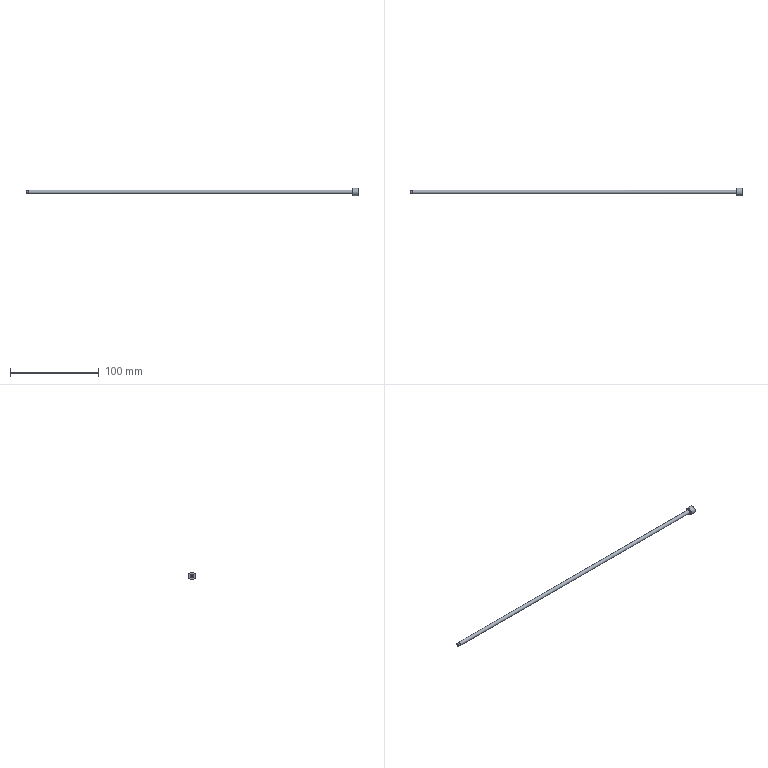Part | STEP file | solid 252 | 1 solid | 7 faces | box 373.765 x 8.5 x 8.5 mm | volume 4948 mm3 | spline 3 | plane 2 | cylinder 2 | commonest cylinder face diameters 4 x1 8.5 x1